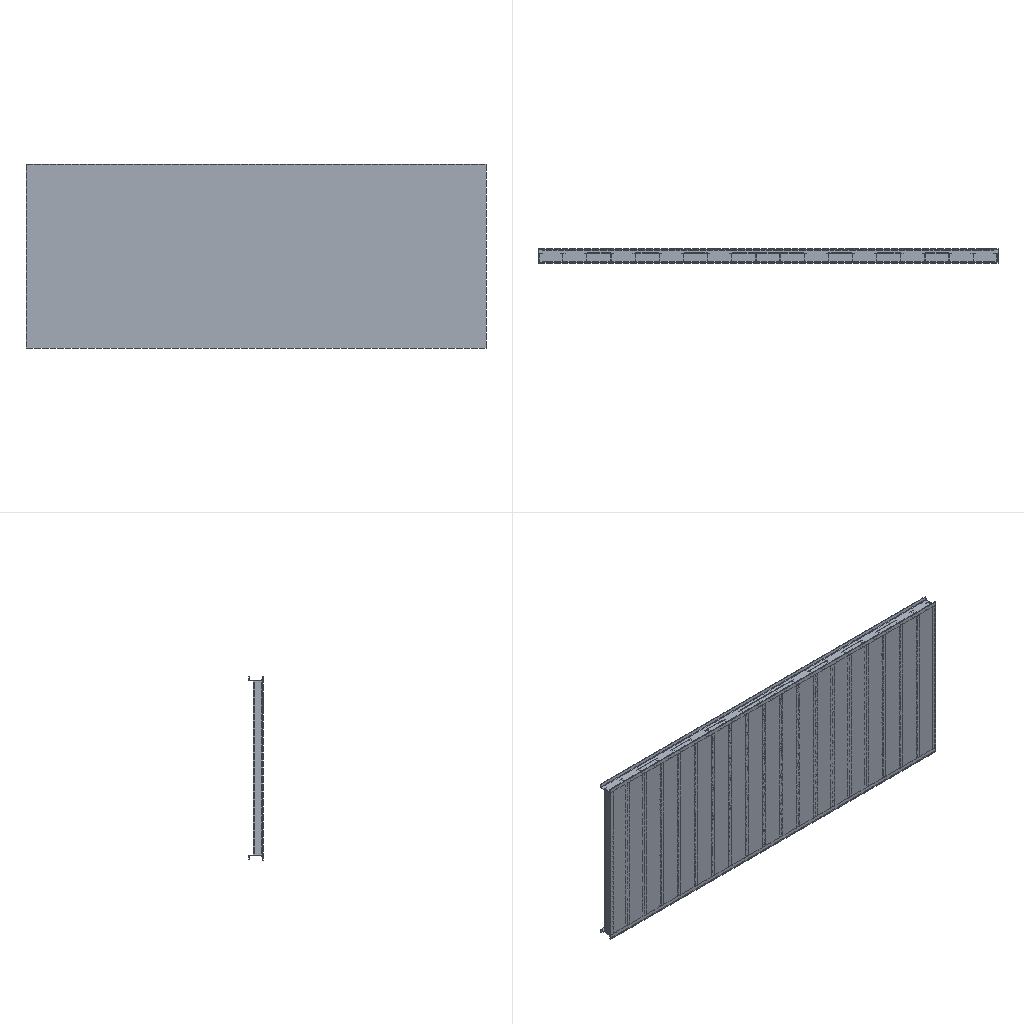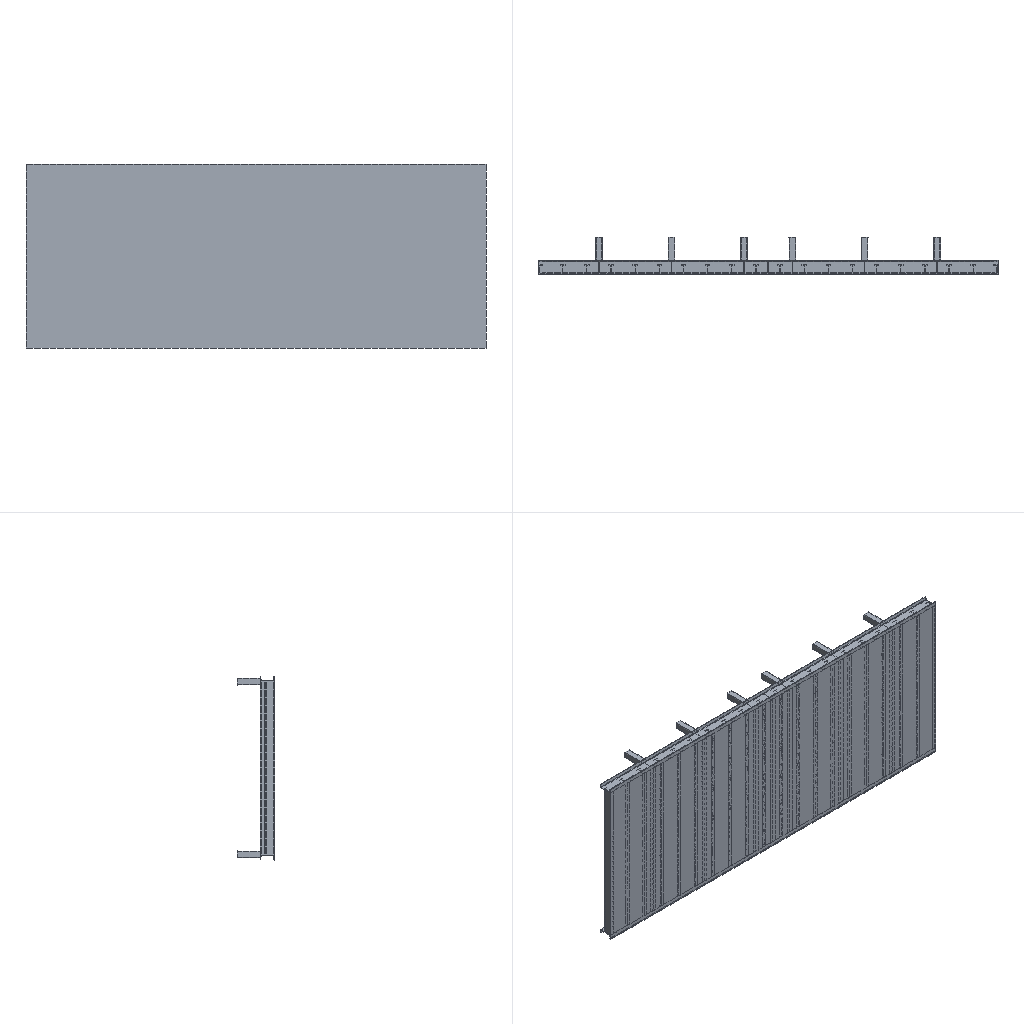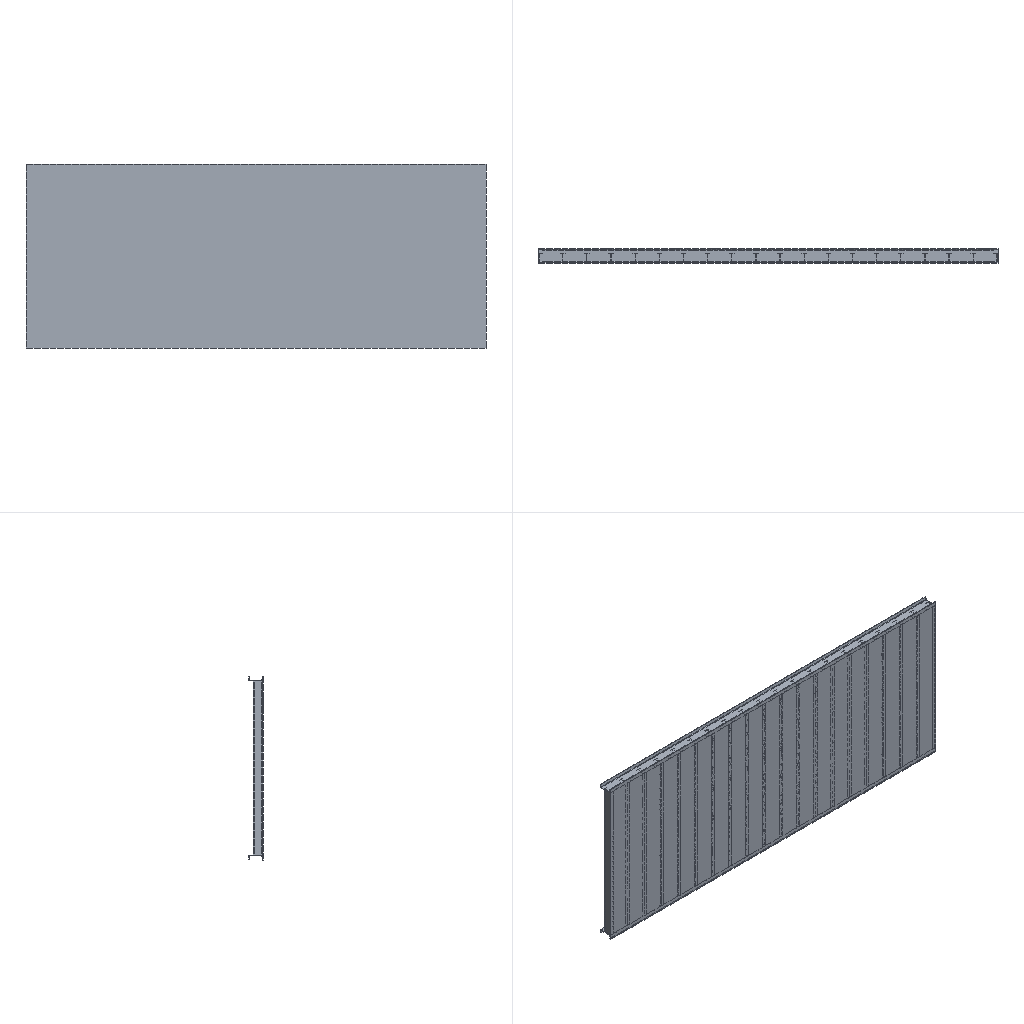Simulation study
Set-up summary, first 218 of 771 lines:
category,name,step,type,value,unit,region
solver,ansys_mapdl
solver,version,,,22.1
solver,version,,,22.1
solver,version,,,22.1
units,MPA,,stated
analysis,deck1,,static,static
load_step,requested,,,1
analysis,nlgeom,,,False
mesh,nodes,,,200363
mesh,elements,,,127797
element_type,ANSYS 187 (type 1),,solid,24917
element_type,ANSYS 187 (type 2),,solid,3615
element_type,ANSYS 187 (type 3),,solid,3615
element_type,ANSYS 187 (type 4),,solid,3615
element_type,ANSYS 187 (type 5),,solid,3615
element_type,ANSYS 187 (type 6),,solid,3615
element_type,ANSYS 187 (type 7),,solid,3615
element_type,ANSYS 187 (type 8),,solid,3615
element_type,ANSYS 187 (type 9),,solid,3615
element_type,ANSYS 187 (type 10),,solid,3615
element_type,ANSYS 187 (type 11),,solid,3615
element_type,ANSYS 187 (type 12),,solid,3615
element_type,ANSYS 187 (type 13),,solid,3615
element_type,ANSYS 187 (type 14),,solid,3615
element_type,ANSYS 187 (type 15),,solid,3615
element_type,ANSYS 187 (type 16),,solid,3615
element_type,ANSYS 187 (type 17),,solid,3615
element_type,ANSYS 187 (type 18),,solid,3053
element_type,ANSYS 187 (type 19),,solid,3615
element_type,ANSYS 187 (type 20),,solid,4163
element_type,ANSYS 187 (type 21),,solid,4163
element_type,ANSYS 186 (type 22),,solid,874
element_type,ANSYS 186 (type 23),,solid,874
element_type,ANSYS 186 (type 24),,solid,24
element_type,ANSYS 186 (type 25),,solid,24
element_type,ANSYS 186 (type 26),,solid,24
element_type,ANSYS 186 (type 27),,solid,24
element_type,ANSYS 186 (type 28),,solid,24
element_type,ANSYS 186 (type 29),,solid,24
element_type,ANSYS 186 (type 30),,solid,24
element_type,ANSYS 186 (type 31),,solid,24
element_type,ANSYS 186 (type 32),,solid,24
element_type,ANSYS 174 (type 33),,contact,395
element_type,ANSYS 170 (type 34),,target,395
element_type,ANSYS 174 (type 35),,contact,405
element_type,ANSYS 170 (type 36),,target,405
element_type,ANSYS 174 (type 37),,contact,393
element_type,ANSYS 170 (type 38),,target,393
element_type,ANSYS 174 (type 39),,contact,391
element_type,ANSYS 170 (type 40),,target,391
element_type,ANSYS 174 (type 41),,contact,427
element_type,ANSYS 170 (type 42),,target,427
element_type,ANSYS 174 (type 43),,contact,407
element_type,ANSYS 170 (type 44),,target,407
element_type,ANSYS 174 (type 45),,contact,383
element_type,ANSYS 170 (type 46),,target,383
element_type,ANSYS 174 (type 47),,contact,411
element_type,ANSYS 170 (type 48),,target,411
element_type,ANSYS 174 (type 49),,contact,410
element_type,ANSYS 170 (type 50),,target,410
element_type,ANSYS 174 (type 51),,contact,394
element_type,ANSYS 170 (type 52),,target,394
element_type,ANSYS 174 (type 53),,contact,407
element_type,ANSYS 170 (type 54),,target,407
element_type,ANSYS 174 (type 55),,contact,386
element_type,ANSYS 170 (type 56),,target,386
element_type,ANSYS 174 (type 57),,contact,411
element_type,ANSYS 170 (type 58),,target,411
element_type,ANSYS 174 (type 59),,contact,417
element_type,ANSYS 170 (type 60),,target,417
element_type,ANSYS 174 (type 61),,contact,386
element_type,ANSYS 170 (type 62),,target,386
element_type,ANSYS 174 (type 63),,contact,410
element_type,ANSYS 170 (type 64),,target,410
element_type,ANSYS 174 (type 65),,contact,358
element_type,ANSYS 170 (type 66),,target,358
element_type,ANSYS 174 (type 67),,contact,406
element_type,ANSYS 170 (type 68),,target,406
element_type,ANSYS 174 (type 69),,contact,668
element_type,ANSYS 170 (type 70),,target,668
element_type,ANSYS 174 (type 71),,contact,660
element_type,ANSYS 170 (type 72),,target,660
element_type,ANSYS 174 (type 73),,contact,213
element_type,ANSYS 170 (type 74),,target,213
element_type,ANSYS 174 (type 75),,contact,211
element_type,ANSYS 170 (type 76),,target,211
element_type,ANSYS 174 (type 77),,contact,38
element_type,ANSYS 170 (type 78),,target,38
element_type,ANSYS 174 (type 79),,contact,38
element_type,ANSYS 170 (type 80),,target,38
element_type,ANSYS 174 (type 81),,contact,40
element_type,ANSYS 170 (type 82),,target,40
element_type,ANSYS 174 (type 83),,contact,40
element_type,ANSYS 170 (type 84),,target,40
element_type,ANSYS 174 (type 85),,contact,38
element_type,ANSYS 170 (type 86),,target,38
element_type,ANSYS 174 (type 87),,contact,38
element_type,ANSYS 170 (type 88),,target,38
element_type,ANSYS 174 (type 89),,contact,38
element_type,ANSYS 170 (type 90),,target,38
element_type,ANSYS 174 (type 91),,contact,38
element_type,ANSYS 170 (type 92),,target,38
element_type,ANSYS 174 (type 93),,contact,38
element_type,ANSYS 170 (type 94),,target,38
element_type,ANSYS 174 (type 95),,contact,38
element_type,ANSYS 170 (type 96),,target,38
element_type,ANSYS 174 (type 97),,contact,40
element_type,ANSYS 170 (type 98),,target,40
element_type,ANSYS 174 (type 99),,contact,40
element_type,ANSYS 170 (type 100),,target,40
element_type,ANSYS 174 (type 101),,contact,38
element_type,ANSYS 170 (type 102),,target,38
element_type,ANSYS 174 (type 103),,contact,38
element_type,ANSYS 170 (type 104),,target,38
element_type,ANSYS 174 (type 105),,contact,38
element_type,ANSYS 170 (type 106),,target,38
element_type,ANSYS 174 (type 107),,contact,38
element_type,ANSYS 170 (type 108),,target,38
element_type,ANSYS 174 (type 109),,contact,38
element_type,ANSYS 170 (type 110),,target,38
element_type,ANSYS 174 (type 111),,contact,38
element_type,ANSYS 170 (type 112),,target,38
element_type,ANSYS 174 (type 113),,contact,40
element_type,ANSYS 170 (type 114),,target,40
element_type,ANSYS 174 (type 115),,contact,40
element_type,ANSYS 170 (type 116),,target,40
element_type,ANSYS 174 (type 117),,contact,38
element_type,ANSYS 170 (type 118),,target,38
element_type,ANSYS 174 (type 119),,contact,38
element_type,ANSYS 170 (type 120),,target,38
element_type,ANSYS 174 (type 121),,contact,38
element_type,ANSYS 170 (type 122),,target,38
element_type,ANSYS 174 (type 123),,contact,38
element_type,ANSYS 170 (type 124),,target,38
element_type,ANSYS 174 (type 125),,contact,38
element_type,ANSYS 170 (type 126),,target,38
element_type,ANSYS 174 (type 127),,contact,38
element_type,ANSYS 170 (type 128),,target,38
element_type,ANSYS 174 (type 129),,contact,40
element_type,ANSYS 170 (type 130),,target,40
element_type,ANSYS 174 (type 131),,contact,40
element_type,ANSYS 170 (type 132),,target,40
element_type,ANSYS 174 (type 133),,contact,38
element_type,ANSYS 170 (type 134),,target,38
element_type,ANSYS 174 (type 135),,contact,38
element_type,ANSYS 170 (type 136),,target,38
element_type,ANSYS 174 (type 137),,contact,38
element_type,ANSYS 170 (type 138),,target,38
element_type,ANSYS 174 (type 139),,contact,38
element_type,ANSYS 170 (type 140),,target,38
element_type,ANSYS 174 (type 141),,contact,40
element_type,ANSYS 170 (type 142),,target,40
element_type,ANSYS 174 (type 143),,contact,40
element_type,ANSYS 170 (type 144),,target,40
element_type,ANSYS 174 (type 145),,contact,40
element_type,ANSYS 170 (type 146),,target,40
element_type,ANSYS 174 (type 147),,contact,40
element_type,ANSYS 170 (type 148),,target,40
element_type,ANSYS 174 (type 149),,contact,37
element_type,ANSYS 170 (type 150),,target,37
element_type,ANSYS 174 (type 151),,contact,40
element_type,ANSYS 170 (type 152),,target,40
element_type,ANSYS 174 (type 153),,contact,40
element_type,ANSYS 170 (type 154),,target,40
element_type,ANSYS 174 (type 155),,contact,37
element_type,ANSYS 170 (type 156),,target,37
element_type,ANSYS 174 (type 157),,contact,134
element_type,ANSYS 170 (type 158),,target,134
element_type,ANSYS 174 (type 159),,contact,134
element_type,ANSYS 170 (type 160),,target,134
element_type,ANSYS 174 (type 161),,contact,134
element_type,ANSYS 170 (type 162),,target,134
element_type,ANSYS 174 (type 163),,contact,134
element_type,ANSYS 170 (type 164),,target,134
element_type,ANSYS 174 (type 165),,contact,134
element_type,ANSYS 170 (type 166),,target,134
element_type,ANSYS 174 (type 167),,contact,134
element_type,ANSYS 170 (type 168),,target,134
element_type,ANSYS 174 (type 169),,contact,134
element_type,ANSYS 170 (type 170),,target,134
element_type,ANSYS 174 (type 171),,contact,134
element_type,ANSYS 170 (type 172),,target,134
element_type,ANSYS 174 (type 173),,contact,134
element_type,ANSYS 170 (type 174),,target,134
element_type,ANSYS 174 (type 175),,contact,134
element_type,ANSYS 170 (type 176),,target,134
element_type,ANSYS 174 (type 177),,contact,134
element_type,ANSYS 170 (type 178),,target,134
element_type,ANSYS 174 (type 179),,contact,134
element_type,ANSYS 170 (type 180),,target,134
element_type,ANSYS 174 (type 181),,contact,134
element_type,ANSYS 170 (type 182),,target,134
element_type,ANSYS 174 (type 183),,contact,134
element_type,ANSYS 170 (type 184),,target,134
element_type,ANSYS 174 (type 185),,contact,134
element_type,ANSYS 170 (type 186),,target,134
element_type,ANSYS 174 (type 187),,contact,134
element_type,ANSYS 170 (type 188),,target,134
element_type,ANSYS 174 (type 189),,contact,134
element_type,ANSYS 170 (type 190),,target,134
element_type,ANSYS 174 (type 191),,contact,109
element_type,ANSYS 170 (type 192),,target,109
element_type,ANSYS 174 (type 193),,contact,30
element_type,ANSYS 170 (type 194),,target,30
element_type,ANSYS 174 (type 195),,contact,30
element_type,ANSYS 170 (type 196),,target,30
element_type,ANSYS 174 (type 197),,contact,30
element_type,ANSYS 170 (type 198),,target,30
element_type,ANSYS 174 (type 199),,contact,30
element_type,ANSYS 170 (type 200),,target,30
element_type,ANSYS 174 (type 201),,contact,31
element_type,ANSYS 170 (type 202),,target,31
element_type,ANSYS 174 (type 203),,contact,30
element_type,ANSYS 170 (type 204),,target,30
element_type,ANSYS 174 (type 205),,contact,31
element_type,ANSYS 170 (type 206),,target,31
element_type,ANSYS 174 (type 207),,contact,30
Results summary:
result,analysis,,,static
result,last_loadstep,,,1
result,primary field,,,displacement
result,reaction total,1,FX,-1.2e-05,N
result,reaction total,1,FY,-550000,N
result,reaction total,1,FZ,66596.914,N
result,mass,,,6.791,"NMM: mm, ton, N, s, mV, mA, degC"
result,analysis,,,static
result,last_loadstep,,,1
result,primary field,,,displacement
result,reaction total,1,FX,-5.9e-05,N
result,reaction total,1,FY,-550000,N
result,reaction total,1,FZ,65308.594,N
result,mass,,,6.66,"NMM: mm, ton, N, s, mV, mA, degC"
result,analysis,,,static
result,last_loadstep,,,1
result,primary field,,,displacement
result,reaction total,1,FX,4.4e-05,N
result,reaction total,1,FY,-550000,N
result,reaction total,1,FZ,53478.021,N
result,mass,,,5.453,"NMM: mm, ton, N, s, mV, mA, degC"